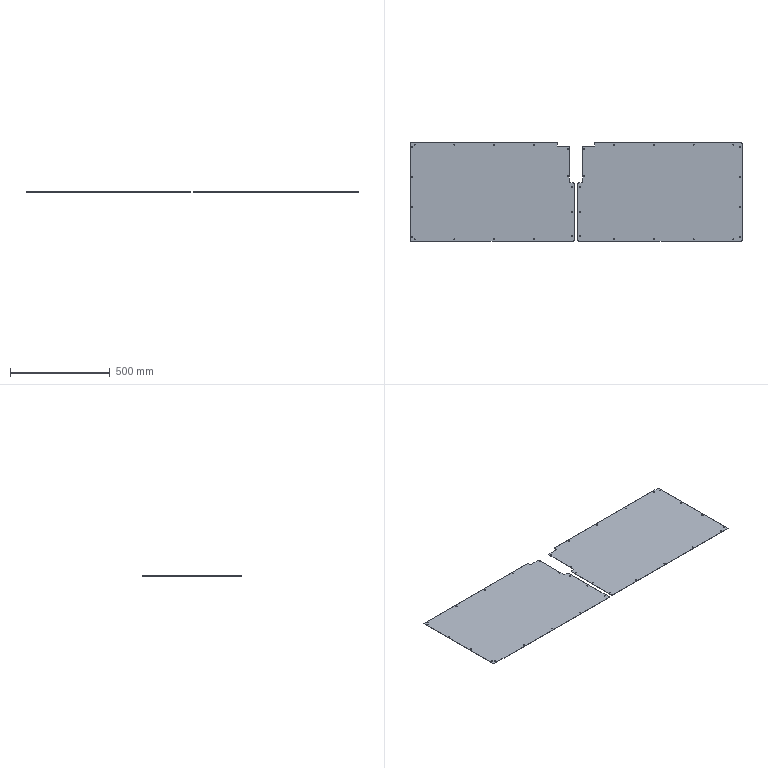Part | NX | features BREP 2 | 2 solids | 102 faces | box 1666 x 496 x 1.5 mm | volume 1205451 mm3 | cylinder 82 | plane 20 | commonest cylinder face diameters 5.5 x68 6 x14